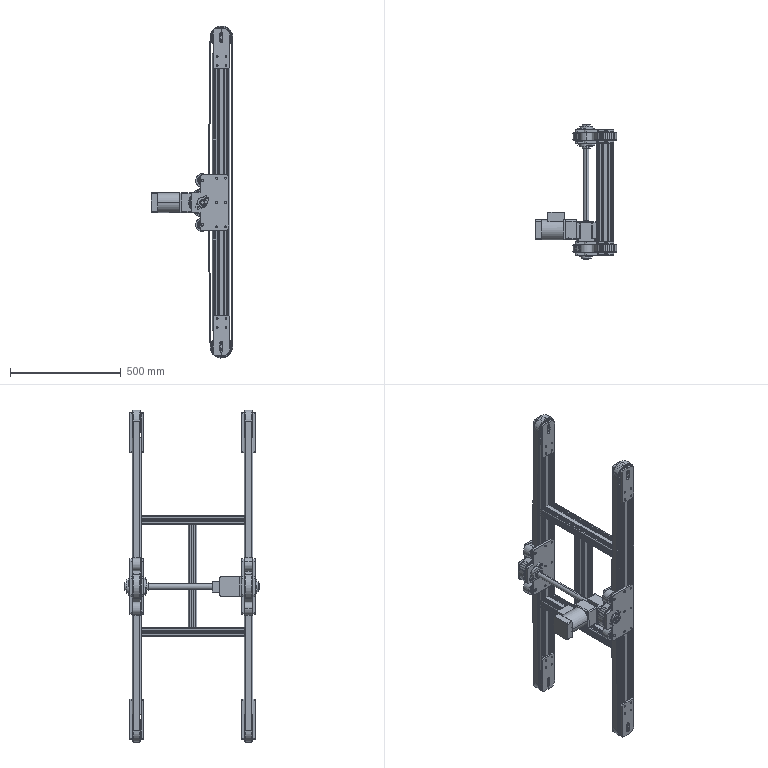Part | SolidWorks | features ReferencePattern 4, MirrorCompFeat 3, CompositeCurve 1, LocalLPattern 1 | 59 solids | 5898 faces | volume 11539429 mm3 | cylinder 2125 | plane 2101 | torus 902 | sphere 512 | spline 144 | cone 114 | commonest cylinder face diameters 1.2 x452 1.6 x452 93.64 x124 2 x102 10 x98 112.74 x72